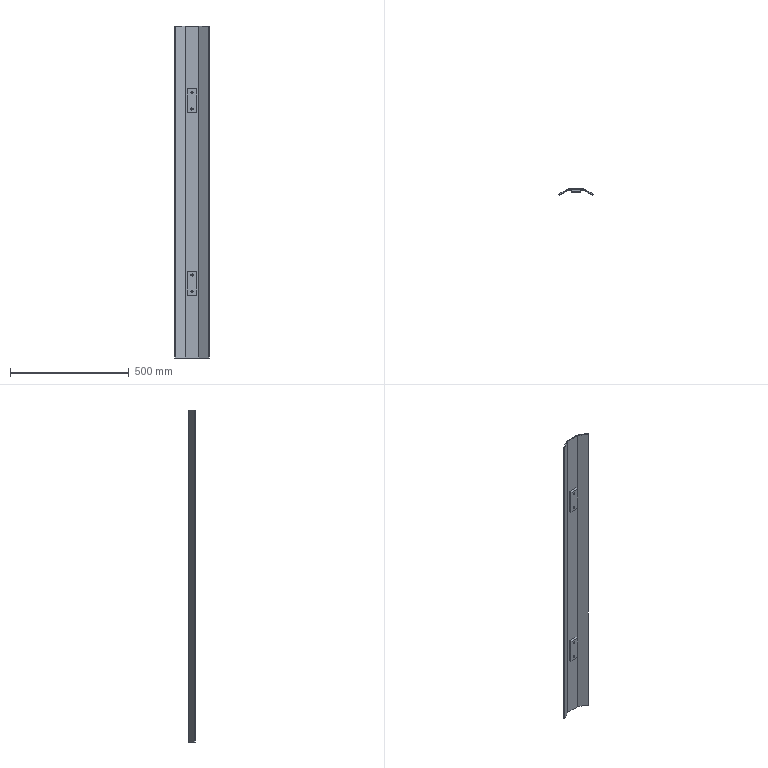Part | STEP file | 3 solids | 42 faces | box 144 x 27.094 x 1400 mm | volume 941168 mm3 | plane 22 | cylinder 20 | commonest cylinder face diameters 8.5 x16 10 x2 18 x2